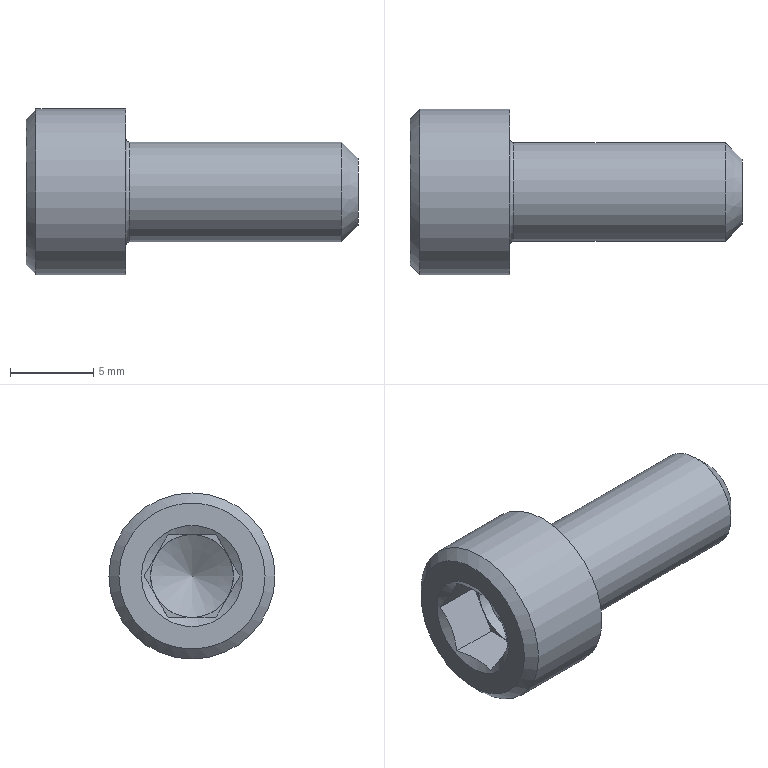Part | STEP file | Винт М6-6gx14 ГОСТ 11738-84 | 1 solid | 23 faces | box 20 x 10 x 10 mm | volume 764.42 mm3 | plane 15 | cone 4 | cylinder 3 | torus 1 | commonest cylinder face diameters 5 x1 6 x1 10 x1
STEP:
#1=CARTESIAN_POINT('',(-6.,4.4,0.));
#2=VERTEX_POINT('',#1);
#3=CARTESIAN_POINT('',(-6.,0.,0.));
#4=DIRECTION('',(1.,0.,0.));
#5=DIRECTION('',(0.,1.,0.));
#6=AXIS2_PLACEMENT_3D('',#3,#4,#5);
#7=CIRCLE('',#6,4.4);
#8=EDGE_CURVE('',#2,#2,#7,.T.);
#9=ORIENTED_EDGE('',*,*,#8,.F.);
#10=EDGE_LOOP('',(#9));
#11=FACE_BOUND('',#10,.T.);
#12=CARTESIAN_POINT('',(-6.,3.05,0.));
#13=VERTEX_POINT('',#12);
#14=CARTESIAN_POINT('',(-6.,0.,0.));
#15=DIRECTION('',(1.,0.,0.));
#16=DIRECTION('',(0.,1.,0.));
#17=AXIS2_PLACEMENT_3D('',#14,#15,#16);
#18=CIRCLE('',#17,3.05);
#19=EDGE_CURVE('',#13,#13,#18,.T.);
#20=ORIENTED_EDGE('',*,*,#19,.T.);
#21=EDGE_LOOP('',(#20));
#22=FACE_BOUND('',#21,.T.);
#23=CARTESIAN_POINT('',(-6.,0.,0.));
#24=DIRECTION('',(-1.,0.,0.));
#25=DIRECTION('',(0.,1.,0.));
#26=AXIS2_PLACEMENT_3D('',#23,#24,#25);
#27=PLANE('',#26);
#28=ADVANCED_FACE('',(#11,#22),#27,.T.);
#29=CARTESIAN_POINT('',(-5.906,1.443,-2.5));
#30=VERTEX_POINT('',#29);
#31=CARTESIAN_POINT('',(-5.906,-1.443,-2.5));
#32=VERTEX_POINT('',#31);
#33=CARTESIAN_POINT('',(-5.906,1.443,-2.5));
#34=CARTESIAN_POINT('',(-5.9,1.424,-2.5));
#35=CARTESIAN_POINT('',(-5.89,1.389,-2.5));
#36=CARTESIAN_POINT('',(-5.88,1.351,-2.5));
#37=CARTESIAN_POINT('',(-5.867,1.304,-2.5));
#38=CARTESIAN_POINT('',(-5.848,1.232,-2.5));
#39=CARTESIAN_POINT('',(-5.827,1.146,-2.5));
#40=CARTESIAN_POINT('',(-5.803,1.043,-2.5));
#41=CARTESIAN_POINT('',(-5.774,0.909,-2.5));
#42=CARTESIAN_POINT('',(-5.75,0.7773,-2.5));
#43=CARTESIAN_POINT('',(-5.728,0.6356,-2.5));
#44=CARTESIAN_POINT('',(-5.711,0.5115,-2.5));
#45=CARTESIAN_POINT('',(-5.699,0.3892,-2.5));
#46=CARTESIAN_POINT('',(-5.692,0.2947,-2.5));
#47=CARTESIAN_POINT('',(-5.688,0.2222,-2.5));
#48=CARTESIAN_POINT('',(-5.684,0.1323,-2.5));
#49=CARTESIAN_POINT('',(-5.683,0.05578,-2.5));
#50=CARTESIAN_POINT('',(-5.682,-0.001577,-2.5));
#51=CARTESIAN_POINT('',(-5.683,-0.03169,-2.5));
#52=CARTESIAN_POINT('',(-5.683,-0.0738,-2.5));
#53=CARTESIAN_POINT('',(-5.684,-0.1276,-2.5));
#54=CARTESIAN_POINT('',(-5.687,-0.2055,-2.5));
#55=CARTESIAN_POINT('',(-5.692,-0.2839,-2.5));
#56=CARTESIAN_POINT('',(-5.696,-0.3444,-2.5));
#57=CARTESIAN_POINT('',(-5.7,-0.3959,-2.5));
#58=CARTESIAN_POINT('',(-5.705,-0.4472,-2.5));
#59=CARTESIAN_POINT('',(-5.713,-0.5148,-2.5));
#60=CARTESIAN_POINT('',(-5.722,-0.5907,-2.5));
#61=CARTESIAN_POINT('',(-5.73,-0.6507,-2.5));
#62=CARTESIAN_POINT('',(-5.738,-0.7005,-2.5));
#63=CARTESIAN_POINT('',(-5.746,-0.7498,-2.5));
#64=CARTESIAN_POINT('',(-5.757,-0.8136,-2.5));
#65=CARTESIAN_POINT('',(-5.77,-0.8864,-2.5));
#66=CARTESIAN_POINT('',(-5.785,-0.9583,-2.5));
#67=CARTESIAN_POINT('',(-5.8,-1.03,-2.5));
#68=CARTESIAN_POINT('',(-5.812,-1.084,-2.5));
#69=CARTESIAN_POINT('',(-5.823,-1.131,-2.5));
#70=CARTESIAN_POINT('',(-5.834,-1.177,-2.5));
#71=CARTESIAN_POINT('',(-5.85,-1.239,-2.5));
#72=CARTESIAN_POINT('',(-5.868,-1.307,-2.5));
#73=CARTESIAN_POINT('',(-5.882,-1.361,-2.5));
#74=CARTESIAN_POINT('',(-5.895,-1.406,-2.5));
#75=CARTESIAN_POINT('',(-5.902,-1.429,-2.5));
#76=CARTESIAN_POINT('',(-5.906,-1.443,-2.5));
#77=B_SPLINE_CURVE_WITH_KNOTS('',3,(#33,#34,#35,#36,#37,#38,#39,#40,#41,#42,#43,#44,#45,#46,#47,#48,#49,#50,#51,#52,#53,#54,#55,#56,#57,#58,#59,#60,#61,#62,#63,#64,#65,#66,#67,#68,#69,#70,#71,#72,#73,#74,#75,#76),.UNSPECIFIED.,.F.,.F.,(4,1,1,1,1,1,1,1,1,1,1,1,1,1,1,1,1,1,1,1,1,1,1,1,1,1,1,1,1,1,1,1,1,1,1,1,1,1,1,1,1,4),(0.,0.02097,0.03685,0.04095,0.07015,0.1134,0.1316,0.1778,0.2541,0.2686,0.3246,0.3823,0.3943,0.4217,0.4566,0.4863,0.5,0.5153,0.5171,0.5431,0.5703,0.5969,0.6234,0.6325,0.6498,0.6761,0.7022,0.7281,0.7381,0.7538,0.7792,0.8044,0.8294,0.8543,0.8789,0.8866,0.9033,0.9276,0.9518,0.9759,0.9843,1.),.UNSPECIFIED.);
#78=EDGE_CURVE('',#30,#32,#77,.T.);
#79=ORIENTED_EDGE('',*,*,#78,.T.);
#80=CARTESIAN_POINT('',(-3.,-1.443,-2.5));
#81=VERTEX_POINT('',#80);
#82=CARTESIAN_POINT('',(-3.,-1.443,-2.5));
#83=DIRECTION('',(-1.,0.,0.));
#84=VECTOR('',#83,1.);
#85=LINE('',#82,#84);
#86=EDGE_CURVE('',#81,#32,#85,.T.);
#87=ORIENTED_EDGE('',*,*,#86,.F.);
#88=CARTESIAN_POINT('',(-3.,0.,-2.5));
#89=VERTEX_POINT('',#88);
#90=CARTESIAN_POINT('',(-3.,0.,-2.5));
#91=DIRECTION('',(0.,-1.,0.));
#92=VECTOR('',#91,1.);
#93=LINE('',#90,#92);
#94=EDGE_CURVE('',#89,#81,#93,.T.);
#95=ORIENTED_EDGE('',*,*,#94,.F.);
#96=CARTESIAN_POINT('',(-3.,1.443,-2.5));
#97=VERTEX_POINT('',#96);
#98=CARTESIAN_POINT('',(-3.,1.443,-2.5));
#99=DIRECTION('',(0.,-1.,0.));
#100=VECTOR('',#99,1.);
#101=LINE('',#98,#100);
#102=EDGE_CURVE('',#97,#89,#101,.T.);
#103=ORIENTED_EDGE('',*,*,#102,.F.);
#104=CARTESIAN_POINT('',(-3.,1.443,-2.5));
#105=DIRECTION('',(-1.,0.,0.));
#106=VECTOR('',#105,1.);
#107=LINE('',#104,#106);
#108=EDGE_CURVE('',#97,#30,#107,.T.);
#109=ORIENTED_EDGE('',*,*,#108,.T.);
#110=EDGE_LOOP('',(#79,#87,#95,#103,#109));
#111=FACE_BOUND('',#110,.T.);
#112=CARTESIAN_POINT('',(-3.,1.443,-2.5));
#113=DIRECTION('',(0.,0.,-1.));
#114=DIRECTION('',(0.,-1.,0.));
#115=AXIS2_PLACEMENT_3D('',#112,#113,#114);
#116=PLANE('',#115);
#117=ADVANCED_FACE('',(#111),#116,.F.);
#118=CARTESIAN_POINT('',(-5.906,-2.887,0.));
#119=VERTEX_POINT('',#118);
#120=CARTESIAN_POINT('',(-5.906,-1.443,-2.5));
#121=CARTESIAN_POINT('',(-5.9,-1.453,-2.483));
#122=CARTESIAN_POINT('',(-5.889,-1.472,-2.45));
#123=CARTESIAN_POINT('',(-5.871,-1.505,-2.392));
#124=CARTESIAN_POINT('',(-5.848,-1.549,-2.317));
#125=CARTESIAN_POINT('',(-5.816,-1.614,-2.204));
#126=CARTESIAN_POINT('',(-5.777,-1.702,-2.052));
#127=CARTESIAN_POINT('',(-5.74,-1.803,-1.877));
#128=CARTESIAN_POINT('',(-5.713,-1.902,-1.705));
#129=CARTESIAN_POINT('',(-5.697,-1.984,-1.564));
#130=CARTESIAN_POINT('',(-5.688,-2.048,-1.453));
#131=CARTESIAN_POINT('',(-5.684,-2.099,-1.365));
#132=CARTESIAN_POINT('',(-5.683,-2.137,-1.298));
#133=CARTESIAN_POINT('',(-5.682,-2.166,-1.249));
#134=CARTESIAN_POINT('',(-5.683,-2.194,-1.201));
#135=CARTESIAN_POINT('',(-5.684,-2.228,-1.141));
#136=CARTESIAN_POINT('',(-5.687,-2.268,-1.072));
#137=CARTESIAN_POINT('',(-5.692,-2.307,-1.004));
#138=CARTESIAN_POINT('',(-5.697,-2.346,-0.9371));
#139=CARTESIAN_POINT('',(-5.704,-2.384,-0.8704));
#140=CARTESIAN_POINT('',(-5.713,-2.422,-0.8041));
#141=CARTESIAN_POINT('',(-5.722,-2.46,-0.7384));
#142=CARTESIAN_POINT('',(-5.733,-2.498,-0.6734));
#143=CARTESIAN_POINT('',(-5.744,-2.535,-0.609));
#144=CARTESIAN_POINT('',(-5.757,-2.572,-0.5454));
#145=CARTESIAN_POINT('',(-5.77,-2.608,-0.4824));
#146=CARTESIAN_POINT('',(-5.785,-2.644,-0.4201));
#147=CARTESIAN_POINT('',(-5.8,-2.68,-0.3584));
#148=CARTESIAN_POINT('',(-5.816,-2.715,-0.2974));
#149=CARTESIAN_POINT('',(-5.832,-2.75,-0.237));
#150=CARTESIAN_POINT('',(-5.85,-2.784,-0.1771));
#151=CARTESIAN_POINT('',(-5.868,-2.819,-0.1177));
#152=CARTESIAN_POINT('',(-5.886,-2.853,-0.05869));
#153=CARTESIAN_POINT('',(-5.899,-2.875,-0.01952));
#154=CARTESIAN_POINT('',(-5.906,-2.887,0.));
#155=B_SPLINE_CURVE_WITH_KNOTS('',3,(#120,#121,#122,#123,#124,#125,#126,#127,#128,#129,#130,#131,#132,#133,#134,#135,#136,#137,#138,#139,#140,#141,#142,#143,#144,#145,#146,#147,#148,#149,#150,#151,#152,#153,#154),.UNSPECIFIED.,.F.,.F.,(4,1,1,1,1,1,1,1,1,1,1,1,1,1,1,1,1,1,1,1,1,1,1,1,1,1,1,1,1,1,1,1,4),(0.,0.02097,0.04095,0.07015,0.1134,0.1778,0.2541,0.3246,0.3823,0.4217,0.4566,0.4863,0.5,0.5153,0.5431,0.5703,0.5969,0.6234,0.6498,0.6761,0.7022,0.7281,0.7538,0.7792,0.8044,0.8294,0.8543,0.8789,0.9033,0.9276,0.9518,0.9759,1.),.UNSPECIFIED.);
#156=EDGE_CURVE('',#32,#119,#155,.T.);
#157=ORIENTED_EDGE('',*,*,#156,.T.);
#158=CARTESIAN_POINT('',(-3.,-2.887,0.));
#159=VERTEX_POINT('',#158);
#160=CARTESIAN_POINT('',(-3.,-2.887,0.));
#161=DIRECTION('',(-1.,0.,0.));
#162=VECTOR('',#161,1.);
#163=LINE('',#160,#162);
#164=EDGE_CURVE('',#159,#119,#163,.T.);
#165=ORIENTED_EDGE('',*,*,#164,.F.);
#166=CARTESIAN_POINT('',(-3.,-2.165,-1.25));
#167=VERTEX_POINT('',#166);
#168=CARTESIAN_POINT('',(-3.,-2.165,-1.25));
#169=DIRECTION('',(0.,-0.5,0.866));
#170=VECTOR('',#169,1.);
#171=LINE('',#168,#170);
#172=EDGE_CURVE('',#167,#159,#171,.T.);
#173=ORIENTED_EDGE('',*,*,#172,.F.);
#174=CARTESIAN_POINT('',(-3.,-1.443,-2.5));
#175=DIRECTION('',(0.,-0.5,0.866));
#176=VECTOR('',#175,1.);
#177=LINE('',#174,#176);
#178=EDGE_CURVE('',#81,#167,#177,.T.);
#179=ORIENTED_EDGE('',*,*,#178,.F.);
#180=ORIENTED_EDGE('',*,*,#86,.T.);
#181=EDGE_LOOP('',(#157,#165,#173,#179,#180));
#182=FACE_BOUND('',#181,.T.);
#183=CARTESIAN_POINT('',(-3.,-1.443,-2.5));
#184=DIRECTION('',(0.,-0.866,-0.5));
#185=DIRECTION('',(0.,-0.5,0.866));
#186=AXIS2_PLACEMENT_3D('',#183,#184,#185);
#187=PLANE('',#186);
#188=ADVANCED_FACE('',(#182),#187,.F.);
#189=CARTESIAN_POINT('',(-5.906,-1.443,2.5));
#190=VERTEX_POINT('',#189);
#191=CARTESIAN_POINT('',(-5.906,-2.887,0.));
#192=CARTESIAN_POINT('',(-5.9,-2.877,0.01704));
#193=CARTESIAN_POINT('',(-5.889,-2.858,0.05036));
#194=CARTESIAN_POINT('',(-5.871,-2.825,0.1076));
#195=CARTESIAN_POINT('',(-5.848,-2.781,0.1832));
#196=CARTESIAN_POINT('',(-5.816,-2.716,0.2956));
#197=CARTESIAN_POINT('',(-5.777,-2.628,0.4476));
#198=CARTESIAN_POINT('',(-5.74,-2.527,0.6235));
#199=CARTESIAN_POINT('',(-5.713,-2.428,0.7948));
#200=CARTESIAN_POINT('',(-5.697,-2.346,0.936));
#201=CARTESIAN_POINT('',(-5.688,-2.282,1.047));
#202=CARTESIAN_POINT('',(-5.684,-2.231,1.135));
#203=CARTESIAN_POINT('',(-5.683,-2.193,1.202));
#204=CARTESIAN_POINT('',(-5.682,-2.164,1.251));
#205=CARTESIAN_POINT('',(-5.683,-2.137,1.299));
#206=CARTESIAN_POINT('',(-5.684,-2.102,1.359));
#207=CARTESIAN_POINT('',(-5.687,-2.062,1.428));
#208=CARTESIAN_POINT('',(-5.692,-2.023,1.496));
#209=CARTESIAN_POINT('',(-5.697,-1.984,1.563));
#210=CARTESIAN_POINT('',(-5.704,-1.946,1.63));
#211=CARTESIAN_POINT('',(-5.713,-1.908,1.696));
#212=CARTESIAN_POINT('',(-5.722,-1.87,1.762));
#213=CARTESIAN_POINT('',(-5.733,-1.832,1.827));
#214=CARTESIAN_POINT('',(-5.744,-1.795,1.891));
#215=CARTESIAN_POINT('',(-5.757,-1.758,1.955));
#216=CARTESIAN_POINT('',(-5.77,-1.722,2.018));
#217=CARTESIAN_POINT('',(-5.785,-1.686,2.08));
#218=CARTESIAN_POINT('',(-5.8,-1.65,2.142));
#219=CARTESIAN_POINT('',(-5.816,-1.615,2.203));
#220=CARTESIAN_POINT('',(-5.832,-1.58,2.263));
#221=CARTESIAN_POINT('',(-5.85,-1.546,2.323));
#222=CARTESIAN_POINT('',(-5.868,-1.511,2.382));
#223=CARTESIAN_POINT('',(-5.886,-1.477,2.441));
#224=CARTESIAN_POINT('',(-5.899,-1.455,2.48));
#225=CARTESIAN_POINT('',(-5.906,-1.443,2.5));
#226=B_SPLINE_CURVE_WITH_KNOTS('',3,(#191,#192,#193,#194,#195,#196,#197,#198,#199,#200,#201,#202,#203,#204,#205,#206,#207,#208,#209,#210,#211,#212,#213,#214,#215,#216,#217,#218,#219,#220,#221,#222,#223,#224,#225),.UNSPECIFIED.,.F.,.F.,(4,1,1,1,1,1,1,1,1,1,1,1,1,1,1,1,1,1,1,1,1,1,1,1,1,1,1,1,1,1,1,1,4),(0.,0.02097,0.04095,0.07015,0.1134,0.1778,0.2541,0.3246,0.3823,0.4217,0.4566,0.4863,0.5,0.5153,0.5431,0.5703,0.5969,0.6234,0.6498,0.6761,0.7022,0.7281,0.7538,0.7792,0.8044,0.8294,0.8543,0.8789,0.9033,0.9276,0.9518,0.9759,1.),.UNSPECIFIED.);
#227=EDGE_CURVE('',#119,#190,#226,.T.);
#228=ORIENTED_EDGE('',*,*,#227,.T.);
#229=CARTESIAN_POINT('',(-3.,-1.443,2.5));
#230=VERTEX_POINT('',#229);
#231=CARTESIAN_POINT('',(-3.,-1.443,2.5));
#232=DIRECTION('',(-1.,0.,0.));
#233=VECTOR('',#232,1.);
#234=LINE('',#231,#233);
#235=EDGE_CURVE('',#230,#190,#234,.T.);
#236=ORIENTED_EDGE('',*,*,#235,.F.);
#237=CARTESIAN_POINT('',(-3.,-2.165,1.25));
#238=VERTEX_POINT('',#237);
#239=CARTESIAN_POINT('',(-3.,-2.165,1.25));
#240=DIRECTION('',(0.,0.5,0.866));
#241=VECTOR('',#240,1.);
#242=LINE('',#239,#241);
#243=EDGE_CURVE('',#238,#230,#242,.T.);
#244=ORIENTED_EDGE('',*,*,#243,.F.);
#245=CARTESIAN_POINT('',(-3.,-2.887,0.));
#246=DIRECTION('',(0.,0.5,0.866));
#247=VECTOR('',#246,1.);
#248=LINE('',#245,#247);
#249=EDGE_CURVE('',#159,#238,#248,.T.);
#250=ORIENTED_EDGE('',*,*,#249,.F.);
#251=ORIENTED_EDGE('',*,*,#164,.T.);
#252=EDGE_LOOP('',(#228,#236,#244,#250,#251));
#253=FACE_BOUND('',#252,.T.);
#254=CARTESIAN_POINT('',(-3.,-2.887,0.));
#255=DIRECTION('',(0.,-0.866,0.5));
#256=DIRECTION('',(0.,0.5,0.866));
#257=AXIS2_PLACEMENT_3D('',#254,#255,#256);
#258=PLANE('',#257);
#259=ADVANCED_FACE('',(#253),#258,.F.);
#260=CARTESIAN_POINT('',(-5.906,1.443,2.5));
#261=VERTEX_POINT('',#260);
#262=CARTESIAN_POINT('',(-5.906,-1.443,2.5));
#263=CARTESIAN_POINT('',(-5.9,-1.424,2.5));
#264=CARTESIAN_POINT('',(-5.89,-1.389,2.5));
#265=CARTESIAN_POINT('',(-5.88,-1.351,2.5));
#266=CARTESIAN_POINT('',(-5.867,-1.304,2.5));
#267=CARTESIAN_POINT('',(-5.848,-1.232,2.5));
#268=CARTESIAN_POINT('',(-5.827,-1.146,2.5));
#269=CARTESIAN_POINT('',(-5.803,-1.043,2.5));
#270=CARTESIAN_POINT('',(-5.774,-0.909,2.5));
#271=CARTESIAN_POINT('',(-5.75,-0.7773,2.5));
#272=CARTESIAN_POINT('',(-5.728,-0.6356,2.5));
#273=CARTESIAN_POINT('',(-5.711,-0.5115,2.5));
#274=CARTESIAN_POINT('',(-5.699,-0.3892,2.5));
#275=CARTESIAN_POINT('',(-5.692,-0.2947,2.5));
#276=CARTESIAN_POINT('',(-5.688,-0.2222,2.5));
#277=CARTESIAN_POINT('',(-5.684,-0.1323,2.5));
#278=CARTESIAN_POINT('',(-5.683,-0.05578,2.5));
#279=CARTESIAN_POINT('',(-5.682,0.001577,2.5));
#280=CARTESIAN_POINT('',(-5.683,0.03169,2.5));
#281=CARTESIAN_POINT('',(-5.683,0.0738,2.5));
#282=CARTESIAN_POINT('',(-5.684,0.1276,2.5));
#283=CARTESIAN_POINT('',(-5.687,0.2055,2.5));
#284=CARTESIAN_POINT('',(-5.692,0.2839,2.5));
#285=CARTESIAN_POINT('',(-5.696,0.3444,2.5));
#286=CARTESIAN_POINT('',(-5.7,0.3959,2.5));
#287=CARTESIAN_POINT('',(-5.705,0.4472,2.5));
#288=CARTESIAN_POINT('',(-5.713,0.5148,2.5));
#289=CARTESIAN_POINT('',(-5.722,0.5907,2.5));
#290=CARTESIAN_POINT('',(-5.73,0.6507,2.5));
#291=CARTESIAN_POINT('',(-5.738,0.7005,2.5));
#292=CARTESIAN_POINT('',(-5.746,0.7498,2.5));
#293=CARTESIAN_POINT('',(-5.757,0.8136,2.5));
#294=CARTESIAN_POINT('',(-5.77,0.8864,2.5));
#295=CARTESIAN_POINT('',(-5.785,0.9583,2.5));
#296=CARTESIAN_POINT('',(-5.8,1.03,2.5));
#297=CARTESIAN_POINT('',(-5.812,1.084,2.5));
#298=CARTESIAN_POINT('',(-5.823,1.131,2.5));
#299=CARTESIAN_POINT('',(-5.834,1.177,2.5));
#300=CARTESIAN_POINT('',(-5.85,1.239,2.5));
#301=CARTESIAN_POINT('',(-5.868,1.307,2.5));
#302=CARTESIAN_POINT('',(-5.882,1.361,2.5));
#303=CARTESIAN_POINT('',(-5.895,1.406,2.5));
#304=CARTESIAN_POINT('',(-5.902,1.429,2.5));
#305=CARTESIAN_POINT('',(-5.906,1.443,2.5));
#306=B_SPLINE_CURVE_WITH_KNOTS('',3,(#262,#263,#264,#265,#266,#267,#268,#269,#270,#271,#272,#273,#274,#275,#276,#277,#278,#279,#280,#281,#282,#283,#284,#285,#286,#287,#288,#289,#290,#291,#292,#293,#294,#295,#296,#297,#298,#299,#300,#301,#302,#303,#304,#305),.UNSPECIFIED.,.F.,.F.,(4,1,1,1,1,1,1,1,1,1,1,1,1,1,1,1,1,1,1,1,1,1,1,1,1,1,1,1,1,1,1,1,1,1,1,1,1,1,1,1,1,4),(0.,0.02097,0.03685,0.04095,0.07015,0.1134,0.1316,0.1778,0.2541,0.2686,0.3246,0.3823,0.3943,0.4217,0.4566,0.4863,0.5,0.5153,0.5171,0.5431,0.5703,0.5969,0.6234,0.6325,0.6498,0.6761,0.7022,0.7281,0.7381,0.7538,0.7792,0.8044,0.8294,0.8543,0.8789,0.8866,0.9033,0.9276,0.9518,0.9759,0.9843,1.),.UNSPECIFIED.);
#307=EDGE_CURVE('',#190,#261,#306,.T.);
#308=ORIENTED_EDGE('',*,*,#307,.T.);
#309=CARTESIAN_POINT('',(-3.,1.443,2.5));
#310=VERTEX_POINT('',#309);
#311=CARTESIAN_POINT('',(-3.,1.443,2.5));
#312=DIRECTION('',(-1.,0.,0.));
#313=VECTOR('',#312,1.);
#314=LINE('',#311,#313);
#315=EDGE_CURVE('',#310,#261,#314,.T.);
#316=ORIENTED_EDGE('',*,*,#315,.F.);
#317=CARTESIAN_POINT('',(-3.,0.,2.5));
#318=VERTEX_POINT('',#317);
#319=CARTESIAN_POINT('',(-3.,0.,2.5));
#320=DIRECTION('',(0.,1.,0.));
#321=VECTOR('',#320,1.);
#322=LINE('',#319,#321);
#323=EDGE_CURVE('',#318,#310,#322,.T.);
#324=ORIENTED_EDGE('',*,*,#323,.F.);
#325=CARTESIAN_POINT('',(-3.,-1.443,2.5));
#326=DIRECTION('',(0.,1.,0.));
#327=VECTOR('',#326,1.);
#328=LINE('',#325,#327);
#329=EDGE_CURVE('',#230,#318,#328,.T.);
#330=ORIENTED_EDGE('',*,*,#329,.F.);
#331=ORIENTED_EDGE('',*,*,#235,.T.);
#332=EDGE_LOOP('',(#308,#316,#324,#330,#331));
#333=FACE_BOUND('',#332,.T.);
#334=CARTESIAN_POINT('',(-3.,-1.443,2.5));
#335=DIRECTION('',(0.,0.,1.));
#336=DIRECTION('',(0.,1.,0.));
#337=AXIS2_PLACEMENT_3D('',#334,#335,#336);
#338=PLANE('',#337);
#339=ADVANCED_FACE('',(#333),#338,.F.);
#340=CARTESIAN_POINT('',(-5.906,2.887,0.));
#341=VERTEX_POINT('',#340);
#342=CARTESIAN_POINT('',(-5.906,2.887,0.));
#343=CARTESIAN_POINT('',(-5.9,2.877,-0.01704));
#344=CARTESIAN_POINT('',(-5.889,2.858,-0.05036));
#345=CARTESIAN_POINT('',(-5.871,2.825,-0.1076));
#346=CARTESIAN_POINT('',(-5.848,2.781,-0.1832));
#347=CARTESIAN_POINT('',(-5.816,2.716,-0.2956));
#348=CARTESIAN_POINT('',(-5.777,2.628,-0.4476));
#349=CARTESIAN_POINT('',(-5.74,2.527,-0.6235));
#350=CARTESIAN_POINT('',(-5.713,2.428,-0.7948));
#351=CARTESIAN_POINT('',(-5.697,2.346,-0.936));
#352=CARTESIAN_POINT('',(-5.688,2.282,-1.047));
#353=CARTESIAN_POINT('',(-5.684,2.231,-1.135));
#354=CARTESIAN_POINT('',(-5.683,2.193,-1.202));
#355=CARTESIAN_POINT('',(-5.682,2.164,-1.251));
#356=CARTESIAN_POINT('',(-5.683,2.137,-1.299));
#357=CARTESIAN_POINT('',(-5.684,2.102,-1.359));
#358=CARTESIAN_POINT('',(-5.687,2.062,-1.428));
#359=CARTESIAN_POINT('',(-5.692,2.023,-1.496));
#360=CARTESIAN_POINT('',(-5.697,1.984,-1.563));
#361=CARTESIAN_POINT('',(-5.704,1.946,-1.63));
#362=CARTESIAN_POINT('',(-5.713,1.908,-1.696));
#363=CARTESIAN_POINT('',(-5.722,1.87,-1.762));
#364=CARTESIAN_POINT('',(-5.733,1.832,-1.827));
#365=CARTESIAN_POINT('',(-5.744,1.795,-1.891));
#366=CARTESIAN_POINT('',(-5.757,1.758,-1.955));
#367=CARTESIAN_POINT('',(-5.77,1.722,-2.018));
#368=CARTESIAN_POINT('',(-5.785,1.686,-2.08));
#369=CARTESIAN_POINT('',(-5.8,1.65,-2.142));
#370=CARTESIAN_POINT('',(-5.816,1.615,-2.203));
#371=CARTESIAN_POINT('',(-5.832,1.58,-2.263));
#372=CARTESIAN_POINT('',(-5.85,1.546,-2.323));
#373=CARTESIAN_POINT('',(-5.868,1.511,-2.382));
#374=CARTESIAN_POINT('',(-5.886,1.477,-2.441));
#375=CARTESIAN_POINT('',(-5.899,1.455,-2.48));
#376=CARTESIAN_POINT('',(-5.906,1.443,-2.5));
#377=B_SPLINE_CURVE_WITH_KNOTS('',3,(#342,#343,#344,#345,#346,#347,#348,#349,#350,#351,#352,#353,#354,#355,#356,#357,#358,#359,#360,#361,#362,#363,#364,#365,#366,#367,#368,#369,#370,#371,#372,#373,#374,#375,#376),.UNSPECIFIED.,.F.,.F.,(4,1,1,1,1,1,1,1,1,1,1,1,1,1,1,1,1,1,1,1,1,1,1,1,1,1,1,1,1,1,1,1,4),(0.,0.02097,0.04095,0.07015,0.1134,0.1778,0.2541,0.3246,0.3823,0.4217,0.4566,0.4863,0.5,0.5153,0.5431,0.5703,0.5969,0.6234,0.6498,0.6761,0.7022,0.7281,0.7538,0.7792,0.8044,0.8294,0.8543,0.8789,0.9033,0.9276,0.9518,0.9759,1.),.UNSPECIFIED.);
#378=EDGE_CURVE('',#341,#30,#377,.T.);
#379=ORIENTED_EDGE('',*,*,#378,.T.);
#380=ORIENTED_EDGE('',*,*,#108,.F.);
#381=CARTESIAN_POINT('',(-3.,2.165,-1.25));
#382=VERTEX_POINT('',#381);
#383=CARTESIAN_POINT('',(-3.,2.165,-1.25));
#384=DIRECTION('',(0.,-0.5,-0.866));
#385=VECTOR('',#384,1.);
#386=LINE('',#383,#385);
#387=EDGE_CURVE('',#382,#97,#386,.T.);
#388=ORIENTED_EDGE('',*,*,#387,.F.);
#389=CARTESIAN_POINT('',(-3.,2.887,0.));
#390=VERTEX_POINT('',#389);
#391=CARTESIAN_POINT('',(-3.,2.887,0.));
#392=DIRECTION('',(0.,-0.5,-0.866));
#393=VECTOR('',#392,1.);
#394=LINE('',#391,#393);
#395=EDGE_CURVE('',#390,#382,#394,.T.);
#396=ORIENTED_EDGE('',*,*,#395,.F.);
#397=CARTESIAN_POINT('',(-3.,2.887,0.));
#398=DIRECTION('',(-1.,0.,0.));
#399=VECTOR('',#398,1.);
#400=LINE('',#397,#399);
#401=EDGE_CURVE('',#390,#341,#400,.T.);
#402=ORIENTED_EDGE('',*,*,#401,.T.);
#403=EDGE_LOOP('',(#379,#380,#388,#396,#402));
#404=FACE_BOUND('',#403,.T.);
#405=CARTESIAN_POINT('',(-3.,2.887,0.));
#406=DIRECTION('',(0.,0.866,-0.5));
#407=DIRECTION('',(0.,-0.5,-0.866));
#408=AXIS2_PLACEMENT_3D('',#405,#406,#407);
#409=PLANE('',#408);
#410=ADVANCED_FACE('',(#404),#409,.F.);
#411=CARTESIAN_POINT('',(-5.906,1.443,2.5));
#412=CARTESIAN_POINT('',(-5.9,1.453,2.483));
#413=CARTESIAN_POINT('',(-5.889,1.472,2.45));
#414=CARTESIAN_POINT('',(-5.871,1.505,2.392));
#415=CARTESIAN_POINT('',(-5.848,1.549,2.317));
#416=CARTESIAN_POINT('',(-5.816,1.614,2.204));
#417=CARTESIAN_POINT('',(-5.777,1.702,2.052));
#418=CARTESIAN_POINT('',(-5.74,1.803,1.877));
#419=CARTESIAN_POINT('',(-5.713,1.902,1.705));
#420=CARTESIAN_POINT('',(-5.697,1.984,1.564));
#421=CARTESIAN_POINT('',(-5.688,2.048,1.453));
#422=CARTESIAN_POINT('',(-5.684,2.099,1.365));
#423=CARTESIAN_POINT('',(-5.683,2.137,1.298));
#424=CARTESIAN_POINT('',(-5.682,2.166,1.249));
#425=CARTESIAN_POINT('',(-5.683,2.194,1.201));
#426=CARTESIAN_POINT('',(-5.684,2.228,1.141));
#427=CARTESIAN_POINT('',(-5.687,2.268,1.072));
#428=CARTESIAN_POINT('',(-5.692,2.307,1.004));
#429=CARTESIAN_POINT('',(-5.697,2.346,0.9371));
#430=CARTESIAN_POINT('',(-5.704,2.384,0.8704));
#431=CARTESIAN_POINT('',(-5.713,2.422,0.8041));
#432=CARTESIAN_POINT('',(-5.722,2.46,0.7384));
#433=CARTESIAN_POINT('',(-5.733,2.498,0.6734));
#434=CARTESIAN_POINT('',(-5.744,2.535,0.609));
#435=CARTESIAN_POINT('',(-5.757,2.572,0.5454));
#436=CARTESIAN_POINT('',(-5.77,2.608,0.4824));
#437=CARTESIAN_POINT('',(-5.785,2.644,0.4201));
#438=CARTESIAN_POINT('',(-5.8,2.68,0.3584));
#439=CARTESIAN_POINT('',(-5.816,2.715,0.2974));
#440=CARTESIAN_POINT('',(-5.832,2.75,0.237));
#441=CARTESIAN_POINT('',(-5.85,2.784,0.1771));
#442=CARTESIAN_POINT('',(-5.868,2.819,0.1177));
#443=CARTESIAN_POINT('',(-5.886,2.853,0.05869));
#444=CARTESIAN_POINT('',(-5.899,2.875,0.01952));
#445=CARTESIAN_POINT('',(-5.906,2.887,0.));
#446=B_SPLINE_CURVE_WITH_KNOTS('',3,(#411,#412,#413,#414,#415,#416,#417,#418,#419,#420,#421,#422,#423,#424,#425,#426,#427,#428,#429,#430,#431,#432,#433,#434,#435,#436,#437,#438,#439,#440,#441,#442,#443,#444,#445),.UNSPECIFIED.,.F.,.F.,(4,1,1,1,1,1,1,1,1,1,1,1,1,1,1,1,1,1,1,1,1,1,1,1,1,1,1,1,1,1,1,1,4),(0.,0.02097,0.04095,0.07015,0.1134,0.1778,0.2541,0.3246,0.3823,0.4217,0.4566,0.4863,0.5,0.5153,0.5431,0.5703,0.5969,0.6234,0.6498,0.6761,0.7022,0.7281,0.7538,0.7792,0.8044,0.8294,0.8543,0.8789,0.9033,0.9276,0.9518,0.9759,1.),.UNSPECIFIED.);
#447=EDGE_CURVE('',#261,#341,#446,.T.);
#448=ORIENTED_EDGE('',*,*,#447,.T.);
#449=ORIENTED_EDGE('',*,*,#401,.F.);
#450=CARTESIAN_POINT('',(-3.,2.165,1.25));
#451=VERTEX_POINT('',#450);
#452=CARTESIAN_POINT('',(-3.,2.165,1.25));
#453=DIRECTION('',(0.,0.5,-0.866));
#454=VECTOR('',#453,1.);
#455=LINE('',#452,#454);
#456=EDGE_CURVE('',#451,#390,#455,.T.);
#457=ORIENTED_EDGE('',*,*,#456,.F.);
#458=CARTESIAN_POINT('',(-3.,1.443,2.5));
#459=DIRECTION('',(0.,0.5,-0.866));
#460=VECTOR('',#459,1.);
#461=LINE('',#458,#460);
#462=EDGE_CURVE('',#310,#451,#461,.T.);
#463=ORIENTED_EDGE('',*,*,#462,.F.);
#464=ORIENTED_EDGE('',*,*,#315,.T.);
#465=EDGE_LOOP('',(#448,#449,#457,#463,#464));
#466=FACE_BOUND('',#465,.T.);
#467=CARTESIAN_POINT('',(-3.,1.443,2.5));
#468=DIRECTION('',(0.,0.866,0.5));
#469=DIRECTION('',(0.,0.5,-0.866));
#470=AXIS2_PLACEMENT_3D('',#467,#468,#469);
#471=PLANE('',#470);
#472=ADVANCED_FACE('',(#466),#471,.F.);
#473=ORIENTED_EDGE('',*,*,#447,.F.);
#474=ORIENTED_EDGE('',*,*,#307,.F.);
#475=ORIENTED_EDGE('',*,*,#227,.F.);
#476=ORIENTED_EDGE('',*,*,#156,.F.);
#477=ORIENTED_EDGE('',*,*,#78,.F.);
#478=ORIENTED_EDGE('',*,*,#378,.F.);
#479=EDGE_LOOP('',(#473,#474,#475,#476,#477,#478));
#480=FACE_BOUND('',#479,.T.);
#481=ORIENTED_EDGE('',*,*,#19,.F.);
#482=EDGE_LOOP('',(#481));
#483=FACE_OUTER_BOUND('',#482,.T.);
#484=CARTESIAN_POINT('',(-5.841,0.,0.));
#485=DIRECTION('',(-1.,0.,0.));
#486=DIRECTION('',(0.,-1.,0.));
#487=AXIS2_PLACEMENT_3D('',#484,#485,#486);
#488=CONICAL_SURFACE('',#487,2.775,1.047);
#489=ADVANCED_FACE('',(#480,#483),#488,.F.);
#490=CARTESIAN_POINT('',(-5.4,5.,0.));
#491=VERTEX_POINT('',#490);
#492=CARTESIAN_POINT('',(-5.4,0.,0.));
#493=DIRECTION('',(1.,0.,0.));
#494=DIRECTION('',(0.,1.,0.));
#495=AXIS2_PLACEMENT_3D('',#492,#493,#494);
#496=CIRCLE('',#495,5.);
#497=EDGE_CURVE('',#491,#491,#496,.T.);
#498=ORIENTED_EDGE('',*,*,#497,.F.);
#499=EDGE_LOOP('',(#498));
#500=FACE_OUTER_BOUND('',#499,.T.);
#501=ORIENTED_EDGE('',*,*,#8,.T.);
#502=EDGE_LOOP('',(#501));
#503=FACE_OUTER_BOUND('',#502,.T.);
#504=CARTESIAN_POINT('',(-5.7,0.,0.));
#505=DIRECTION('',(1.,0.,0.));
#506=DIRECTION('',(0.,1.,0.));
#507=AXIS2_PLACEMENT_3D('',#504,#505,#506);
#508=CONICAL_SURFACE('',#507,4.7,0.7854);
#509=ADVANCED_FACE('',(#500,#503),#508,.T.);
#510=CARTESIAN_POINT('',(-3.,0.,0.));
#511=DIRECTION('',(1.,0.,0.));
#512=DIRECTION('',(0.,-0.866,-0.5));
#513=AXIS2_PLACEMENT_3D('',#510,#511,#512);
#514=CIRCLE('',#513,2.5);
#515=EDGE_CURVE('',#167,#89,#514,.T.);
#516=ORIENTED_EDGE('',*,*,#515,.T.);
#517=ORIENTED_EDGE('',*,*,#94,.T.);
#518=ORIENTED_EDGE('',*,*,#178,.T.);
#519=EDGE_LOOP('',(#516,#517,#518));
#520=FACE_BOUND('',#519,.T.);
#521=CARTESIAN_POINT('',(-3.,0.,0.));
#522=DIRECTION('',(-1.,0.,0.));
#523=DIRECTION('',(0.,0.,-1.));
#524=AXIS2_PLACEMENT_3D('',#521,#522,#523);
#525=PLANE('',#524);
#526=ADVANCED_FACE('',(#520),#525,.T.);
#527=CARTESIAN_POINT('',(-3.,0.,0.));
#528=DIRECTION('',(1.,0.,0.));
#529=DIRECTION('',(0.,0.,-1.));
#530=AXIS2_PLACEMENT_3D('',#527,#528,#529);
#531=CIRCLE('',#530,2.5);
#532=EDGE_CURVE('',#89,#382,#531,.T.);
#533=ORIENTED_EDGE('',*,*,#532,.T.);
#534=ORIENTED_EDGE('',*,*,#387,.T.);
#535=ORIENTED_EDGE('',*,*,#102,.T.);
#536=EDGE_LOOP('',(#533,#534,#535));
#537=FACE_BOUND('',#536,.T.);
#538=CARTESIAN_POINT('',(-3.,0.,0.));
#539=DIRECTION('',(-1.,0.,0.));
#540=DIRECTION('',(0.,0.,-1.));
#541=AXIS2_PLACEMENT_3D('',#538,#539,#540);
#542=PLANE('',#541);
#543=ADVANCED_FACE('',(#537),#542,.T.);
#544=CARTESIAN_POINT('',(-3.,0.,0.));
#545=DIRECTION('',(1.,0.,0.));
#546=DIRECTION('',(0.,-0.866,0.5));
#547=AXIS2_PLACEMENT_3D('',#544,#545,#546);
#548=CIRCLE('',#547,2.5);
#549=EDGE_CURVE('',#238,#167,#548,.T.);
#550=ORIENTED_EDGE('',*,*,#549,.T.);
#551=ORIENTED_EDGE('',*,*,#172,.T.);
#552=ORIENTED_EDGE('',*,*,#249,.T.);
#553=EDGE_LOOP('',(#550,#551,#552));
#554=FACE_BOUND('',#553,.T.);
#555=CARTESIAN_POINT('',(-3.,0.,0.));
#556=DIRECTION('',(-1.,0.,0.));
#557=DIRECTION('',(0.,0.,-1.));
#558=AXIS2_PLACEMENT_3D('',#555,#556,#557);
#559=PLANE('',#558);
#560=ADVANCED_FACE('',(#554),#559,.T.);
#561=CARTESIAN_POINT('',(-3.,0.,0.));
#562=DIRECTION('',(1.,0.,0.));
#563=DIRECTION('',(0.,0.,1.));
#564=AXIS2_PLACEMENT_3D('',#561,#562,#563);
#565=CIRCLE('',#564,2.5);
#566=EDGE_CURVE('',#318,#238,#565,.T.);
#567=ORIENTED_EDGE('',*,*,#566,.T.);
#568=ORIENTED_EDGE('',*,*,#243,.T.);
#569=ORIENTED_EDGE('',*,*,#329,.T.);
#570=EDGE_LOOP('',(#567,#568,#569));
#571=FACE_BOUND('',#570,.T.);
#572=CARTESIAN_POINT('',(-3.,0.,0.));
#573=DIRECTION('',(-1.,0.,0.));
#574=DIRECTION('',(0.,0.,-1.));
#575=AXIS2_PLACEMENT_3D('',#572,#573,#574);
#576=PLANE('',#575);
#577=ADVANCED_FACE('',(#571),#576,.T.);
#578=CARTESIAN_POINT('',(-3.,0.,0.));
#579=DIRECTION('',(1.,0.,0.));
#580=DIRECTION('',(0.,0.866,0.5));
#581=AXIS2_PLACEMENT_3D('',#578,#579,#580);
#582=CIRCLE('',#581,2.5);
#583=EDGE_CURVE('',#451,#318,#582,.T.);
#584=ORIENTED_EDGE('',*,*,#583,.T.);
#585=ORIENTED_EDGE('',*,*,#323,.T.);
#586=ORIENTED_EDGE('',*,*,#462,.T.);
#587=EDGE_LOOP('',(#584,#585,#586));
#588=FACE_BOUND('',#587,.T.);
#589=CARTESIAN_POINT('',(-3.,0.,0.));
#590=DIRECTION('',(-1.,0.,0.));
#591=DIRECTION('',(0.,0.,-1.));
#592=AXIS2_PLACEMENT_3D('',#589,#590,#591);
#593=PLANE('',#592);
#594=ADVANCED_FACE('',(#588),#593,.T.);
#595=CARTESIAN_POINT('',(-3.,2.5,0.));
#596=VERTEX_POINT('',#595);
#597=CARTESIAN_POINT('',(-3.,0.,0.));
#598=DIRECTION('',(1.,0.,0.));
#599=DIRECTION('',(0.,1.,0.));
#600=AXIS2_PLACEMENT_3D('',#597,#598,#599);
#601=CIRCLE('',#600,2.5);
#602=EDGE_CURVE('',#596,#451,#601,.T.);
#603=ORIENTED_EDGE('',*,*,#602,.T.);
#604=ORIENTED_EDGE('',*,*,#456,.T.);
#605=ORIENTED_EDGE('',*,*,#395,.T.);
#606=CARTESIAN_POINT('',(-3.,0.,0.));
#607=DIRECTION('',(1.,0.,0.));
#608=DIRECTION('',(0.,0.866,-0.5));
#609=AXIS2_PLACEMENT_3D('',#606,#607,#608);
#610=CIRCLE('',#609,2.5);
#611=EDGE_CURVE('',#382,#596,#610,.T.);
#612=ORIENTED_EDGE('',*,*,#611,.T.);
#613=EDGE_LOOP('',(#603,#604,#605,#612));
#614=FACE_BOUND('',#613,.T.);
#615=CARTESIAN_POINT('',(-3.,0.,0.));
#616=DIRECTION('',(-1.,0.,0.));
#617=DIRECTION('',(0.,0.,-1.));
#618=AXIS2_PLACEMENT_3D('',#615,#616,#617);
#619=PLANE('',#618);
#620=ADVANCED_FACE('',(#614),#619,.T.);
#621=CARTESIAN_POINT('',(0.,5.,0.));
#622=VERTEX_POINT('',#621);
#623=CARTESIAN_POINT('',(0.,0.,0.));
#624=DIRECTION('',(1.,0.,0.));
#625=DIRECTION('',(0.,1.,0.));
#626=AXIS2_PLACEMENT_3D('',#623,#624,#625);
#627=CIRCLE('',#626,5.);
#628=EDGE_CURVE('',#622,#622,#627,.T.);
#629=ORIENTED_EDGE('',*,*,#628,.F.);
#630=EDGE_LOOP('',(#629));
#631=FACE_OUTER_BOUND('',#630,.T.);
#632=ORIENTED_EDGE('',*,*,#497,.T.);
#633=EDGE_LOOP('',(#632));
#634=FACE_OUTER_BOUND('',#633,.T.);
#635=CARTESIAN_POINT('',(-6.,0.,0.));
#636=DIRECTION('',(1.,0.,0.));
#637=DIRECTION('',(0.,1.,0.));
#638=AXIS2_PLACEMENT_3D('',#635,#636,#637);
#639=CYLINDRICAL_SURFACE('',#638,5.);
#640=ADVANCED_FACE('',(#631,#634),#639,.T.);
#641=CARTESIAN_POINT('',(-2.3,2.5,0.));
#642=VERTEX_POINT('',#641);
#643=CARTESIAN_POINT('',(-2.3,0.,0.));
#644=DIRECTION('',(1.,0.,0.));
#645=DIRECTION('',(0.,1.,0.));
#646=AXIS2_PLACEMENT_3D('',#643,#644,#645);
#647=CIRCLE('',#646,2.5);
#648=EDGE_CURVE('',#642,#642,#647,.T.);
#649=ORIENTED_EDGE('',*,*,#648,.T.);
#650=EDGE_LOOP('',(#649));
#651=FACE_OUTER_BOUND('',#650,.T.);
#652=ORIENTED_EDGE('',*,*,#611,.F.);
#653=ORIENTED_EDGE('',*,*,#532,.F.);
#654=ORIENTED_EDGE('',*,*,#515,.F.);
#655=ORIENTED_EDGE('',*,*,#549,.F.);
#656=ORIENTED_EDGE('',*,*,#566,.F.);
#657=ORIENTED_EDGE('',*,*,#583,.F.);
#658=ORIENTED_EDGE('',*,*,#602,.F.);
#659=EDGE_LOOP('',(#652,#653,#654,#655,#656,#657,#658));
#660=FACE_BOUND('',#659,.T.);
#661=CARTESIAN_POINT('',(-6.,0.,0.));
#662=DIRECTION('',(1.,0.,0.));
#663=DIRECTION('',(0.,1.,0.));
#664=AXIS2_PLACEMENT_3D('',#661,#662,#663);
#665=CYLINDRICAL_SURFACE('',#664,2.5);
#666=ADVANCED_FACE('',(#651,#660),#665,.F.);
#667=ORIENTED_EDGE('',*,*,#628,.T.);
#668=EDGE_LOOP('',(#667));
#669=FACE_BOUND('',#668,.T.);
#670=CARTESIAN_POINT('',(0.,0.,-3.25));
#671=VERTEX_POINT('',#670);
#672=CARTESIAN_POINT('',(0.,0.,0.));
#673=DIRECTION('',(-1.,0.,0.));
#674=DIRECTION('',(0.,0.,-1.));
#675=AXIS2_PLACEMENT_3D('',#672,#673,#674);
#676=CIRCLE('',#675,3.25);
#677=EDGE_CURVE('',#671,#671,#676,.T.);
#678=ORIENTED_EDGE('',*,*,#677,.T.);
#679=EDGE_LOOP('',(#678));
#680=FACE_BOUND('',#679,.T.);
#681=CARTESIAN_POINT('',(0.,0.,0.));
#682=DIRECTION('',(1.,0.,0.));
#683=DIRECTION('',(0.,1.,0.));
#684=AXIS2_PLACEMENT_3D('',#681,#682,#683);
#685=PLANE('',#684);
#686=ADVANCED_FACE('',(#669,#680),#685,.T.);
#687=ORIENTED_EDGE('',*,*,#648,.F.);
#688=EDGE_LOOP('',(#687));
#689=FACE_OUTER_BOUND('',#688,.T.);
#690=CARTESIAN_POINT('',(-1.578,0.,0.));
#691=DIRECTION('',(-1.,0.,0.));
#692=DIRECTION('',(0.,-1.,0.));
#693=AXIS2_PLACEMENT_3D('',#690,#691,#692);
#694=CONICAL_SURFACE('',#693,1.25,1.047);
#695=ADVANCED_FACE('',(#689),#694,.F.);
#696=CARTESIAN_POINT('',(0.25,0.,-3.));
#697=VERTEX_POINT('',#696);
#698=CARTESIAN_POINT('',(0.25,0.,0.));
#699=DIRECTION('',(-1.,0.,0.));
#700=DIRECTION('',(0.,0.,-1.));
#701=AXIS2_PLACEMENT_3D('',#698,#699,#700);
#702=CIRCLE('',#701,3.);
#703=EDGE_CURVE('',#697,#697,#702,.T.);
#704=ORIENTED_EDGE('',*,*,#703,.T.);
#705=EDGE_LOOP('',(#704));
#706=FACE_OUTER_BOUND('',#705,.T.);
#707=ORIENTED_EDGE('',*,*,#677,.F.);
#708=EDGE_LOOP('',(#707));
#709=FACE_OUTER_BOUND('',#708,.T.);
#710=CARTESIAN_POINT('',(0.25,0.,0.));
#711=DIRECTION('',(-1.,0.,0.));
#712=DIRECTION('',(0.,0.,-1.));
#713=AXIS2_PLACEMENT_3D('',#710,#711,#712);
#714=TOROIDAL_SURFACE('',#713,3.25,0.25);
#715=ADVANCED_FACE('',(#706,#709),#714,.F.);
#716=CARTESIAN_POINT('',(13.,0.,-3.));
#717=VERTEX_POINT('',#716);
#718=CARTESIAN_POINT('',(13.,0.,0.));
#719=DIRECTION('',(-1.,0.,0.));
#720=DIRECTION('',(0.,0.,-1.));
#721=AXIS2_PLACEMENT_3D('',#718,#719,#720);
#722=CIRCLE('',#721,3.);
#723=EDGE_CURVE('',#717,#717,#722,.T.);
#724=ORIENTED_EDGE('',*,*,#723,.T.);
#725=EDGE_LOOP('',(#724));
#726=FACE_OUTER_BOUND('',#725,.T.);
#727=ORIENTED_EDGE('',*,*,#703,.F.);
#728=EDGE_LOOP('',(#727));
#729=FACE_OUTER_BOUND('',#728,.T.);
#730=CARTESIAN_POINT('',(14.,0.,0.));
#731=DIRECTION('',(-1.,0.,0.));
#732=DIRECTION('',(0.,0.,-1.));
#733=AXIS2_PLACEMENT_3D('',#730,#731,#732);
#734=CYLINDRICAL_SURFACE('',#733,3.);
#735=ADVANCED_FACE('',(#726,#729),#734,.T.);
#736=CARTESIAN_POINT('',(14.,0.,-2.));
#737=VERTEX_POINT('',#736);
#738=CARTESIAN_POINT('',(14.,0.,0.));
#739=DIRECTION('',(-1.,0.,0.));
#740=DIRECTION('',(0.,0.,-1.));
#741=AXIS2_PLACEMENT_3D('',#738,#739,#740);
#742=CIRCLE('',#741,2.);
#743=EDGE_CURVE('',#737,#737,#742,.T.);
#744=ORIENTED_EDGE('',*,*,#743,.F.);
#745=EDGE_LOOP('',(#744));
#746=FACE_BOUND('',#745,.T.);
#747=CARTESIAN_POINT('',(14.,0.,0.));
#748=DIRECTION('',(-1.,0.,0.));
#749=DIRECTION('',(0.,0.,-1.));
#750=AXIS2_PLACEMENT_3D('',#747,#748,#749);
#751=PLANE('',#750);
#752=ADVANCED_FACE('',(#746),#751,.F.);
#753=ORIENTED_EDGE('',*,*,#743,.T.);
#754=EDGE_LOOP('',(#753));
#755=FACE_OUTER_BOUND('',#754,.T.);
#756=ORIENTED_EDGE('',*,*,#723,.F.);
#757=EDGE_LOOP('',(#756));
#758=FACE_OUTER_BOUND('',#757,.T.);
#759=CARTESIAN_POINT('',(13.5,0.,0.));
#760=DIRECTION('',(-1.,0.,0.));
#761=DIRECTION('',(0.,0.,-1.));
#762=AXIS2_PLACEMENT_3D('',#759,#760,#761);
#763=CONICAL_SURFACE('',#762,2.5,0.7854);
#764=ADVANCED_FACE('',(#755,#758),#763,.T.);
#765=CLOSED_SHELL('',(#28,#117,#188,#259,#339,#410,#472,#489,#509,#526,#543,#560,#577,#594,#620,#640,#666,#686,#695,#715,#735,#752,#764));
#766=MANIFOLD_SOLID_BREP('',#765);
#767=(LENGTH_UNIT()NAMED_UNIT(*)SI_UNIT(.MILLI.,.METRE.));
#768=UNCERTAINTY_MEASURE_WITH_UNIT(LENGTH_MEASURE(0.00001),#767,'','');
#769=(NAMED_UNIT(*)PLANE_ANGLE_UNIT()SI_UNIT($,.RADIAN.));
#770=(NAMED_UNIT(*)SI_UNIT($,.STERADIAN.)SOLID_ANGLE_UNIT());
#771=(GEOMETRIC_REPRESENTATION_CONTEXT(3)GLOBAL_UNCERTAINTY_ASSIGNED_CONTEXT((#768))GLOBAL_UNIT_ASSIGNED_CONTEXT((#767,#769,#770))REPRESENTATION_CONTEXT('',''));
#772=ADVANCED_BREP_SHAPE_REPRESENTATION('',(#766),#771);